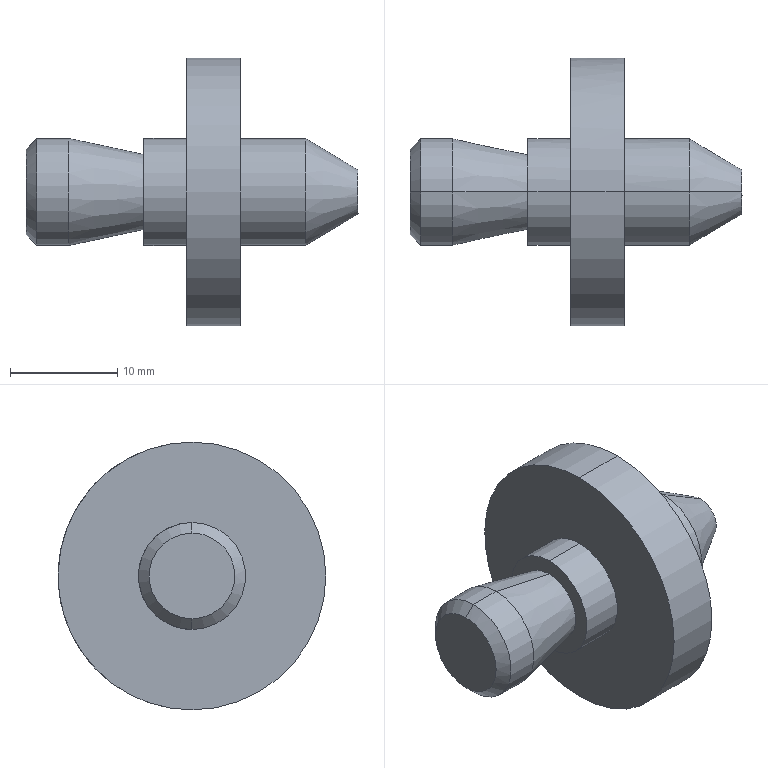Part | STEP file | Positioning_id38_x_t | 1 solid | 19 faces | box 31 x 25 x 25 mm | volume 4152 mm3 | cylinder 8 | cone 6 | plane 5 | commonest cylinder face diameters 10 x6 25 x2
STEP:
#1=CARTESIAN_POINT('',(0.,0.,0.));
#2=DIRECTION('',(0.,0.,1.));
#3=DIRECTION('',(1.,0.,0.));
#4=AXIS2_PLACEMENT_3D('',#1,#2,#3);
#5=CARTESIAN_POINT('',(-829.886,0.00006182,198.532));
#6=VERTEX_POINT('',#5);
#7=CARTESIAN_POINT('',(-824.999,0.00006182,195.6));
#8=VERTEX_POINT('',#7);
#9=CARTESIAN_POINT('',(-824.999,0.00006182,195.6));
#10=DIRECTION('',(0.8575,0.,-0.5145));
#11=VECTOR('',#10,1.);
#12=LINE('',#9,#11);
#13=CARTESIAN_POINT('',(-832.028,0.00006182,193.532));
#14=DIRECTION('',(-1.,0.,0.));
#15=DIRECTION('',(0.,0.,1.));
#16=AXIS2_PLACEMENT_3D('',#13,#14,#15);
#17=CONICAL_SURFACE('',#16,6.285,0.5404);
#18=CARTESIAN_POINT('',(0.,-7.029));
#19=DIRECTION('',(0.,-1.));
#20=VECTOR('',#19,1.);
#21=LINE('',#18,#20);
#22=(GEOMETRIC_REPRESENTATION_CONTEXT(2)PARAMETRIC_REPRESENTATION_CONTEXT()REPRESENTATION_CONTEXT('',''));
#23=DEFINITIONAL_REPRESENTATION('',(#21),#22);
#24=PCURVE('',#17,#23);
#25=CARTESIAN_POINT('',(-832.028,0.00006182,193.532));
#26=DIRECTION('',(-1.,0.,0.));
#27=DIRECTION('',(0.,0.,1.));
#28=AXIS2_PLACEMENT_3D('',#25,#26,#27);
#29=CONICAL_SURFACE('',#28,6.285,0.5404);
#30=CARTESIAN_POINT('',(6.283,-7.029));
#31=DIRECTION('',(0.,-1.));
#32=VECTOR('',#31,1.);
#33=LINE('',#30,#32);
#34=(GEOMETRIC_REPRESENTATION_CONTEXT(2)PARAMETRIC_REPRESENTATION_CONTEXT()REPRESENTATION_CONTEXT('',''));
#35=DEFINITIONAL_REPRESENTATION('',(#33),#34);
#36=PCURVE('',#29,#35);
#37=SURFACE_CURVE('',#12,(#24,#36),.PCURVE_S1.);
#38=EDGE_CURVE('',#6,#8,#37,.T.);
#39=ORIENTED_EDGE('',*,*,#38,.T.);
#40=CARTESIAN_POINT('',(-824.999,0.00006182,191.464));
#41=VERTEX_POINT('',#40);
#42=CARTESIAN_POINT('',(-824.999,0.00006182,193.532));
#43=DIRECTION('',(1.,0.,0.));
#44=DIRECTION('',(0.,0.,1.));
#45=AXIS2_PLACEMENT_3D('',#42,#43,#44);
#46=CIRCLE('',#45,2.068);
#47=CARTESIAN_POINT('',(6.283,-7.029));
#48=DIRECTION('',(-1.,0.));
#49=VECTOR('',#48,1.);
#50=LINE('',#47,#49);
#51=(GEOMETRIC_REPRESENTATION_CONTEXT(2)PARAMETRIC_REPRESENTATION_CONTEXT()REPRESENTATION_CONTEXT('',''));
#52=DEFINITIONAL_REPRESENTATION('',(#50),#51);
#53=PCURVE('',#17,#52);
#54=CARTESIAN_POINT('',(-824.999,0.00006182,193.532));
#55=DIRECTION('',(1.,0.,0.));
#56=DIRECTION('',(0.,0.,1.));
#57=AXIS2_PLACEMENT_3D('',#54,#55,#56);
#58=PLANE('',#57);
#59=CARTESIAN_POINT('',(0.,0.));
#60=DIRECTION('',(1.,0.));
#61=AXIS2_PLACEMENT_2D('',#59,#60);
#62=CIRCLE('',#61,2.068);
#63=(GEOMETRIC_REPRESENTATION_CONTEXT(2)PARAMETRIC_REPRESENTATION_CONTEXT()REPRESENTATION_CONTEXT('',''));
#64=DEFINITIONAL_REPRESENTATION('',(#62),#63);
#65=PCURVE('',#58,#64);
#66=SURFACE_CURVE('',#46,(#53,#65),.PCURVE_S1.);
#67=EDGE_CURVE('',#41,#8,#66,.T.);
#68=ORIENTED_EDGE('',*,*,#67,.F.);
#69=CARTESIAN_POINT('',(-829.886,0.00006182,188.532));
#70=VERTEX_POINT('',#69);
#71=CARTESIAN_POINT('',(-824.999,0.00006182,191.464));
#72=DIRECTION('',(-0.8575,0.,-0.5145));
#73=VECTOR('',#72,1.);
#74=LINE('',#71,#73);
#75=CARTESIAN_POINT('',(3.142,-7.029));
#76=DIRECTION('',(0.,1.));
#77=VECTOR('',#76,1.);
#78=LINE('',#75,#77);
#79=(GEOMETRIC_REPRESENTATION_CONTEXT(2)PARAMETRIC_REPRESENTATION_CONTEXT()REPRESENTATION_CONTEXT('',''));
#80=DEFINITIONAL_REPRESENTATION('',(#78),#79);
#81=PCURVE('',#17,#80);
#82=CARTESIAN_POINT('',(3.142,-7.029));
#83=DIRECTION('',(0.,1.));
#84=VECTOR('',#83,1.);
#85=LINE('',#82,#84);
#86=(GEOMETRIC_REPRESENTATION_CONTEXT(2)PARAMETRIC_REPRESENTATION_CONTEXT()REPRESENTATION_CONTEXT('',''));
#87=DEFINITIONAL_REPRESENTATION('',(#85),#86);
#88=PCURVE('',#29,#87);
#89=SURFACE_CURVE('',#74,(#81,#88),.PCURVE_S1.);
#90=EDGE_CURVE('',#41,#70,#89,.T.);
#91=ORIENTED_EDGE('',*,*,#90,.T.);
#92=CARTESIAN_POINT('',(-829.886,0.00006182,193.532));
#93=DIRECTION('',(-1.,0.,0.));
#94=DIRECTION('',(0.,0.,1.));
#95=AXIS2_PLACEMENT_3D('',#92,#93,#94);
#96=CIRCLE('',#95,5.);
#97=CARTESIAN_POINT('',(0.,-2.142));
#98=DIRECTION('',(1.,0.));
#99=VECTOR('',#98,1.);
#100=LINE('',#97,#99);
#101=(GEOMETRIC_REPRESENTATION_CONTEXT(2)PARAMETRIC_REPRESENTATION_CONTEXT()REPRESENTATION_CONTEXT('',''));
#102=DEFINITIONAL_REPRESENTATION('',(#100),#101);
#103=PCURVE('',#17,#102);
#104=CARTESIAN_POINT('',(-835.999,0.00006182,193.532));
#105=DIRECTION('',(-1.,0.,0.));
#106=DIRECTION('',(0.,0.,1.));
#107=AXIS2_PLACEMENT_3D('',#104,#105,#106);
#108=CYLINDRICAL_SURFACE('',#107,5.);
#109=CARTESIAN_POINT('',(0.,-6.113));
#110=DIRECTION('',(1.,0.));
#111=VECTOR('',#110,1.);
#112=LINE('',#109,#111);
#113=(GEOMETRIC_REPRESENTATION_CONTEXT(2)PARAMETRIC_REPRESENTATION_CONTEXT()REPRESENTATION_CONTEXT('',''));
#114=DEFINITIONAL_REPRESENTATION('',(#112),#113);
#115=PCURVE('',#108,#114);
#116=SURFACE_CURVE('',#96,(#103,#115),.PCURVE_S1.);
#117=EDGE_CURVE('',#6,#70,#116,.T.);
#118=ORIENTED_EDGE('',*,*,#117,.F.);
#119=EDGE_LOOP('',(#39,#68,#91,#118));
#120=FACE_BOUND('',#119,.T.);
#121=ADVANCED_FACE('',(#120),#17,.T.);
#122=CARTESIAN_POINT('',(-835.999,0.00006182,198.532));
#123=VERTEX_POINT('',#122);
#124=CARTESIAN_POINT('',(-835.999,0.00006182,198.532));
#125=DIRECTION('',(1.,0.,0.));
#126=VECTOR('',#125,1.);
#127=LINE('',#124,#126);
#128=CARTESIAN_POINT('',(-835.999,0.00006182,193.532));
#129=DIRECTION('',(-1.,0.,0.));
#130=DIRECTION('',(0.,0.,1.));
#131=AXIS2_PLACEMENT_3D('',#128,#129,#130);
#132=CYLINDRICAL_SURFACE('',#131,5.);
#133=CARTESIAN_POINT('',(6.283,0.));
#134=DIRECTION('',(0.,-1.));
#135=VECTOR('',#134,1.);
#136=LINE('',#133,#135);
#137=(GEOMETRIC_REPRESENTATION_CONTEXT(2)PARAMETRIC_REPRESENTATION_CONTEXT()REPRESENTATION_CONTEXT('',''));
#138=DEFINITIONAL_REPRESENTATION('',(#136),#137);
#139=PCURVE('',#132,#138);
#140=CARTESIAN_POINT('',(0.,0.));
#141=DIRECTION('',(0.,-1.));
#142=VECTOR('',#141,1.);
#143=LINE('',#140,#142);
#144=(GEOMETRIC_REPRESENTATION_CONTEXT(2)PARAMETRIC_REPRESENTATION_CONTEXT()REPRESENTATION_CONTEXT('',''));
#145=DEFINITIONAL_REPRESENTATION('',(#143),#144);
#146=PCURVE('',#108,#145);
#147=SURFACE_CURVE('',#127,(#139,#146),.PCURVE_S1.);
#148=EDGE_CURVE('',#123,#6,#147,.T.);
#149=ORIENTED_EDGE('',*,*,#148,.F.);
#150=CARTESIAN_POINT('',(-835.999,0.00006182,188.532));
#151=VERTEX_POINT('',#150);
#152=CARTESIAN_POINT('',(-835.999,0.00006182,193.532));
#153=DIRECTION('',(1.,0.,0.));
#154=DIRECTION('',(0.,0.,1.));
#155=AXIS2_PLACEMENT_3D('',#152,#153,#154);
#156=CIRCLE('',#155,5.);
#157=CARTESIAN_POINT('',(6.283,0.));
#158=DIRECTION('',(-1.,0.));
#159=VECTOR('',#158,1.);
#160=LINE('',#157,#159);
#161=(GEOMETRIC_REPRESENTATION_CONTEXT(2)PARAMETRIC_REPRESENTATION_CONTEXT()REPRESENTATION_CONTEXT('',''));
#162=DEFINITIONAL_REPRESENTATION('',(#160),#161);
#163=PCURVE('',#132,#162);
#164=CARTESIAN_POINT('',(-835.999,0.00006182,193.532));
#165=DIRECTION('',(1.,0.,0.));
#166=DIRECTION('',(0.,0.,1.));
#167=AXIS2_PLACEMENT_3D('',#164,#165,#166);
#168=PLANE('',#167);
#169=CARTESIAN_POINT('',(0.,0.));
#170=DIRECTION('',(1.,0.));
#171=AXIS2_PLACEMENT_2D('',#169,#170);
#172=CIRCLE('',#171,5.);
#173=(GEOMETRIC_REPRESENTATION_CONTEXT(2)PARAMETRIC_REPRESENTATION_CONTEXT()REPRESENTATION_CONTEXT('',''));
#174=DEFINITIONAL_REPRESENTATION('',(#172),#173);
#175=PCURVE('',#168,#174);
#176=SURFACE_CURVE('',#156,(#163,#175),.PCURVE_S1.);
#177=EDGE_CURVE('',#123,#151,#176,.T.);
#178=ORIENTED_EDGE('',*,*,#177,.T.);
#179=CARTESIAN_POINT('',(-835.999,0.00006182,188.532));
#180=DIRECTION('',(-1.,0.,0.));
#181=VECTOR('',#180,1.);
#182=LINE('',#179,#181);
#183=CARTESIAN_POINT('',(3.142,0.));
#184=DIRECTION('',(0.,1.));
#185=VECTOR('',#184,1.);
#186=LINE('',#183,#185);
#187=(GEOMETRIC_REPRESENTATION_CONTEXT(2)PARAMETRIC_REPRESENTATION_CONTEXT()REPRESENTATION_CONTEXT('',''));
#188=DEFINITIONAL_REPRESENTATION('',(#186),#187);
#189=PCURVE('',#132,#188);
#190=CARTESIAN_POINT('',(3.142,0.));
#191=DIRECTION('',(0.,1.));
#192=VECTOR('',#191,1.);
#193=LINE('',#190,#192);
#194=(GEOMETRIC_REPRESENTATION_CONTEXT(2)PARAMETRIC_REPRESENTATION_CONTEXT()REPRESENTATION_CONTEXT('',''));
#195=DEFINITIONAL_REPRESENTATION('',(#193),#194);
#196=PCURVE('',#108,#195);
#197=SURFACE_CURVE('',#182,(#189,#196),.PCURVE_S1.);
#198=EDGE_CURVE('',#70,#151,#197,.T.);
#199=ORIENTED_EDGE('',*,*,#198,.F.);
#200=CARTESIAN_POINT('',(-829.886,0.00006182,193.532));
#201=DIRECTION('',(-1.,0.,0.));
#202=DIRECTION('',(0.,0.,-1.));
#203=AXIS2_PLACEMENT_3D('',#200,#201,#202);
#204=CIRCLE('',#203,5.);
#205=CARTESIAN_POINT('',(3.142,-6.113));
#206=DIRECTION('',(1.,0.));
#207=VECTOR('',#206,1.);
#208=LINE('',#205,#207);
#209=(GEOMETRIC_REPRESENTATION_CONTEXT(2)PARAMETRIC_REPRESENTATION_CONTEXT()REPRESENTATION_CONTEXT('',''));
#210=DEFINITIONAL_REPRESENTATION('',(#208),#209);
#211=PCURVE('',#132,#210);
#212=CARTESIAN_POINT('',(3.142,-2.142));
#213=DIRECTION('',(1.,0.));
#214=VECTOR('',#213,1.);
#215=LINE('',#212,#214);
#216=(GEOMETRIC_REPRESENTATION_CONTEXT(2)PARAMETRIC_REPRESENTATION_CONTEXT()REPRESENTATION_CONTEXT('',''));
#217=DEFINITIONAL_REPRESENTATION('',(#215),#216);
#218=PCURVE('',#29,#217);
#219=SURFACE_CURVE('',#204,(#211,#218),.PCURVE_S1.);
#220=EDGE_CURVE('',#70,#6,#219,.T.);
#221=ORIENTED_EDGE('',*,*,#220,.T.);
#222=EDGE_LOOP('',(#149,#178,#199,#221));
#223=FACE_BOUND('',#222,.T.);
#224=ADVANCED_FACE('',(#223),#132,.T.);
#225=ORIENTED_EDGE('',*,*,#67,.T.);
#226=CARTESIAN_POINT('',(-824.999,0.00006182,195.6));
#227=CARTESIAN_POINT('',(-824.999,-2.068,195.6));
#228=CARTESIAN_POINT('',(-824.999,-3.101,193.532));
#229=CARTESIAN_POINT('',(-824.999,-2.068,191.464));
#230=CARTESIAN_POINT('',(-824.999,0.00006182,191.464));
#231=(BOUNDED_CURVE()B_SPLINE_CURVE(4,(#226,#227,#228,#229,#230),.UNSPECIFIED.,.F.,.F.)B_SPLINE_CURVE_WITH_KNOTS((5,5),(0.,1.),.PIECEWISE_BEZIER_KNOTS.)CURVE()GEOMETRIC_REPRESENTATION_ITEM()RATIONAL_B_SPLINE_CURVE((1.,0.7071,0.6667,0.7071,1.))REPRESENTATION_ITEM(''));
#232=CARTESIAN_POINT('',(2.068,0.));
#233=CARTESIAN_POINT('',(2.068,2.068));
#234=CARTESIAN_POINT('',(0.,3.101));
#235=CARTESIAN_POINT('',(-2.068,2.068));
#236=CARTESIAN_POINT('',(-2.068,0.));
#237=(BOUNDED_CURVE()B_SPLINE_CURVE(4,(#232,#233,#234,#235,#236),.UNSPECIFIED.,.F.,.F.)B_SPLINE_CURVE_WITH_KNOTS((5,5),(0.,1.),.PIECEWISE_BEZIER_KNOTS.)CURVE()GEOMETRIC_REPRESENTATION_ITEM()RATIONAL_B_SPLINE_CURVE((1.,0.7071,0.6667,0.7071,1.))REPRESENTATION_ITEM(''));
#238=(GEOMETRIC_REPRESENTATION_CONTEXT(2)PARAMETRIC_REPRESENTATION_CONTEXT()REPRESENTATION_CONTEXT('',''));
#239=DEFINITIONAL_REPRESENTATION('',(#237),#238);
#240=PCURVE('',#58,#239);
#241=CARTESIAN_POINT('',(6.283,-7.029));
#242=CARTESIAN_POINT('',(6.24,-7.029));
#243=CARTESIAN_POINT('',(6.153,-7.029));
#244=CARTESIAN_POINT('',(6.02,-7.029));
#245=CARTESIAN_POINT('',(5.883,-7.029));
#246=CARTESIAN_POINT('',(5.744,-7.029));
#247=CARTESIAN_POINT('',(5.602,-7.029));
#248=CARTESIAN_POINT('',(5.457,-7.029));
#249=CARTESIAN_POINT('',(5.311,-7.029));
#250=CARTESIAN_POINT('',(5.163,-7.029));
#251=CARTESIAN_POINT('',(5.013,-7.029));
#252=CARTESIAN_POINT('',(4.863,-7.029));
#253=CARTESIAN_POINT('',(4.712,-7.029));
#254=CARTESIAN_POINT('',(4.562,-7.029));
#255=CARTESIAN_POINT('',(4.412,-7.029));
#256=CARTESIAN_POINT('',(4.262,-7.029));
#257=CARTESIAN_POINT('',(4.114,-7.029));
#258=CARTESIAN_POINT('',(3.968,-7.029));
#259=CARTESIAN_POINT('',(3.823,-7.029));
#260=CARTESIAN_POINT('',(3.681,-7.029));
#261=CARTESIAN_POINT('',(3.542,-7.029));
#262=CARTESIAN_POINT('',(3.405,-7.029));
#263=CARTESIAN_POINT('',(3.271,-7.029));
#264=CARTESIAN_POINT('',(3.184,-7.029));
#265=CARTESIAN_POINT('',(3.142,-7.029));
#266=B_SPLINE_CURVE_WITH_KNOTS('',3,(#241,#242,#243,#244,#245,#246,#247,#248,#249,#250,#251,#252,#253,#254,#255,#256,#257,#258,#259,#260,#261,#262,#263,#264,#265),.UNSPECIFIED.,.F.,.F.,(4,1,1,1,1,1,1,1,1,1,1,1,1,1,1,1,1,1,1,1,1,1,4),(0.,0.04545,0.09091,0.1364,0.1818,0.2273,0.2727,0.3182,0.3636,0.4091,0.4545,0.5,0.5455,0.5909,0.6364,0.6818,0.7273,0.7727,0.8182,0.8636,0.9091,0.9545,1.),.QUASI_UNIFORM_KNOTS.);
#267=(GEOMETRIC_REPRESENTATION_CONTEXT(2)PARAMETRIC_REPRESENTATION_CONTEXT()REPRESENTATION_CONTEXT('',''));
#268=DEFINITIONAL_REPRESENTATION('',(#266),#267);
#269=PCURVE('',#29,#268);
#270=SURFACE_CURVE('',#231,(#240,#269),.PCURVE_S1.);
#271=EDGE_CURVE('',#8,#41,#270,.T.);
#272=ORIENTED_EDGE('',*,*,#271,.T.);
#273=EDGE_LOOP('',(#225,#272));
#274=FACE_BOUND('',#273,.T.);
#275=ADVANCED_FACE('',(#274),#58,.T.);
#276=CARTESIAN_POINT('',(-844.999,0.00006182,190.032));
#277=VERTEX_POINT('',#276);
#278=CARTESIAN_POINT('',(-844.999,0.00006182,197.032));
#279=VERTEX_POINT('',#278);
#280=CARTESIAN_POINT('',(-844.999,0.00006182,193.532));
#281=DIRECTION('',(1.,0.,0.));
#282=DIRECTION('',(0.,0.,-1.));
#283=AXIS2_PLACEMENT_3D('',#280,#281,#282);
#284=CIRCLE('',#283,3.5);
#285=CARTESIAN_POINT('',(-844.999,0.00006182,193.532));
#286=DIRECTION('',(1.,0.,0.));
#287=DIRECTION('',(0.,0.,1.));
#288=AXIS2_PLACEMENT_3D('',#285,#286,#287);
#289=PLANE('',#288);
#290=CARTESIAN_POINT('',(0.,0.));
#291=DIRECTION('',(-1.,0.));
#292=AXIS2_PLACEMENT_2D('',#290,#291);
#293=CIRCLE('',#292,3.5);
#294=(GEOMETRIC_REPRESENTATION_CONTEXT(2)PARAMETRIC_REPRESENTATION_CONTEXT()REPRESENTATION_CONTEXT('',''));
#295=DEFINITIONAL_REPRESENTATION('',(#293),#294);
#296=PCURVE('',#289,#295);
#297=CARTESIAN_POINT('',(-851.999,0.00006182,193.532));
#298=DIRECTION('',(-1.,0.,0.));
#299=DIRECTION('',(0.,0.,1.));
#300=AXIS2_PLACEMENT_3D('',#297,#298,#299);
#301=CONICAL_SURFACE('',#300,5.,0.2111);
#302=CARTESIAN_POINT('',(3.142,-7.));
#303=DIRECTION('',(-1.,0.));
#304=VECTOR('',#303,1.);
#305=LINE('',#302,#304);
#306=(GEOMETRIC_REPRESENTATION_CONTEXT(2)PARAMETRIC_REPRESENTATION_CONTEXT()REPRESENTATION_CONTEXT('',''));
#307=DEFINITIONAL_REPRESENTATION('',(#305),#306);
#308=PCURVE('',#301,#307);
#309=SURFACE_CURVE('',#284,(#296,#308),.PCURVE_S1.);
#310=EDGE_CURVE('',#277,#279,#309,.T.);
#311=ORIENTED_EDGE('',*,*,#310,.T.);
#312=CARTESIAN_POINT('',(-844.999,0.00006182,193.532));
#313=DIRECTION('',(1.,0.,0.));
#314=DIRECTION('',(0.,0.,1.));
#315=AXIS2_PLACEMENT_3D('',#312,#313,#314);
#316=CIRCLE('',#315,3.5);
#317=CARTESIAN_POINT('',(0.,0.));
#318=DIRECTION('',(1.,0.));
#319=AXIS2_PLACEMENT_2D('',#317,#318);
#320=CIRCLE('',#319,3.5);
#321=(GEOMETRIC_REPRESENTATION_CONTEXT(2)PARAMETRIC_REPRESENTATION_CONTEXT()REPRESENTATION_CONTEXT('',''));
#322=DEFINITIONAL_REPRESENTATION('',(#320),#321);
#323=PCURVE('',#289,#322);
#324=CARTESIAN_POINT('',(-851.999,0.00006182,193.532));
#325=DIRECTION('',(-1.,0.,0.));
#326=DIRECTION('',(0.,0.,1.));
#327=AXIS2_PLACEMENT_3D('',#324,#325,#326);
#328=CONICAL_SURFACE('',#327,5.,0.2111);
#329=CARTESIAN_POINT('',(6.283,-7.));
#330=DIRECTION('',(-1.,0.));
#331=VECTOR('',#330,1.);
#332=LINE('',#329,#331);
#333=(GEOMETRIC_REPRESENTATION_CONTEXT(2)PARAMETRIC_REPRESENTATION_CONTEXT()REPRESENTATION_CONTEXT('',''));
#334=DEFINITIONAL_REPRESENTATION('',(#332),#333);
#335=PCURVE('',#328,#334);
#336=SURFACE_CURVE('',#316,(#323,#335),.PCURVE_S1.);
#337=EDGE_CURVE('',#279,#277,#336,.T.);
#338=ORIENTED_EDGE('',*,*,#337,.T.);
#339=EDGE_LOOP('',(#311,#338));
#340=FACE_BOUND('',#339,.T.);
#341=CARTESIAN_POINT('',(-844.999,0.00006182,188.532));
#342=VERTEX_POINT('',#341);
#343=CARTESIAN_POINT('',(-844.999,0.00006182,198.532));
#344=VERTEX_POINT('',#343);
#345=CARTESIAN_POINT('',(-844.999,0.00006182,193.532));
#346=DIRECTION('',(-1.,0.,0.));
#347=DIRECTION('',(0.,0.,-1.));
#348=AXIS2_PLACEMENT_3D('',#345,#346,#347);
#349=CIRCLE('',#348,5.);
#350=CARTESIAN_POINT('',(-5.,0.));
#351=CARTESIAN_POINT('',(-5.,8.66));
#352=CARTESIAN_POINT('',(2.5,4.33));
#353=CARTESIAN_POINT('',(10.,0.));
#354=CARTESIAN_POINT('',(2.5,-4.33));
#355=CARTESIAN_POINT('',(-5.,-8.66));
#356=CARTESIAN_POINT('',(-5.,0.));
#357=(BOUNDED_CURVE()B_SPLINE_CURVE(2,(#350,#351,#352,#353,#354,#355,#356),.UNSPECIFIED.,.T.,.F.)B_SPLINE_CURVE_WITH_KNOTS((1,2,2,2,2,1),(-2.094,0.,2.094,4.189,6.283,8.378),.UNSPECIFIED.)CURVE()GEOMETRIC_REPRESENTATION_ITEM()RATIONAL_B_SPLINE_CURVE((1.,0.5,1.,0.5,1.,0.5,1.))REPRESENTATION_ITEM(''));
#358=(GEOMETRIC_REPRESENTATION_CONTEXT(2)PARAMETRIC_REPRESENTATION_CONTEXT()REPRESENTATION_CONTEXT('',''));
#359=DEFINITIONAL_REPRESENTATION('',(#357),#358);
#360=PCURVE('',#289,#359);
#361=CARTESIAN_POINT('',(-845.999,0.00006182,193.532));
#362=DIRECTION('',(-1.,0.,0.));
#363=DIRECTION('',(0.,0.,1.));
#364=AXIS2_PLACEMENT_3D('',#361,#362,#363);
#365=CYLINDRICAL_SURFACE('',#364,5.);
#366=CARTESIAN_POINT('',(3.142,-1.));
#367=DIRECTION('',(1.,0.));
#368=VECTOR('',#367,1.);
#369=LINE('',#366,#368);
#370=(GEOMETRIC_REPRESENTATION_CONTEXT(2)PARAMETRIC_REPRESENTATION_CONTEXT()REPRESENTATION_CONTEXT('',''));
#371=DEFINITIONAL_REPRESENTATION('',(#369),#370);
#372=PCURVE('',#365,#371);
#373=SURFACE_CURVE('',#349,(#360,#372),.PCURVE_S1.);
#374=EDGE_CURVE('',#342,#344,#373,.T.);
#375=ORIENTED_EDGE('',*,*,#374,.T.);
#376=CARTESIAN_POINT('',(-844.999,0.00006182,193.532));
#377=DIRECTION('',(-1.,0.,0.));
#378=DIRECTION('',(0.,0.,1.));
#379=AXIS2_PLACEMENT_3D('',#376,#377,#378);
#380=CIRCLE('',#379,5.);
#381=CARTESIAN_POINT('',(5.,0.));
#382=CARTESIAN_POINT('',(5.,-8.66));
#383=CARTESIAN_POINT('',(-2.5,-4.33));
#384=CARTESIAN_POINT('',(-10.,0.));
#385=CARTESIAN_POINT('',(-2.5,4.33));
#386=CARTESIAN_POINT('',(5.,8.66));
#387=CARTESIAN_POINT('',(5.,0.));
#388=(BOUNDED_CURVE()B_SPLINE_CURVE(2,(#381,#382,#383,#384,#385,#386,#387),.UNSPECIFIED.,.T.,.F.)B_SPLINE_CURVE_WITH_KNOTS((1,2,2,2,2,1),(-2.094,0.,2.094,4.189,6.283,8.378),.UNSPECIFIED.)CURVE()GEOMETRIC_REPRESENTATION_ITEM()RATIONAL_B_SPLINE_CURVE((1.,0.5,1.,0.5,1.,0.5,1.))REPRESENTATION_ITEM(''));
#389=(GEOMETRIC_REPRESENTATION_CONTEXT(2)PARAMETRIC_REPRESENTATION_CONTEXT()REPRESENTATION_CONTEXT('',''));
#390=DEFINITIONAL_REPRESENTATION('',(#388),#389);
#391=PCURVE('',#289,#390);
#392=CARTESIAN_POINT('',(-845.999,0.00006182,193.532));
#393=DIRECTION('',(-1.,0.,0.));
#394=DIRECTION('',(0.,0.,1.));
#395=AXIS2_PLACEMENT_3D('',#392,#393,#394);
#396=CYLINDRICAL_SURFACE('',#395,5.);
#397=CARTESIAN_POINT('',(0.,-1.));
#398=DIRECTION('',(1.,0.));
#399=VECTOR('',#398,1.);
#400=LINE('',#397,#399);
#401=(GEOMETRIC_REPRESENTATION_CONTEXT(2)PARAMETRIC_REPRESENTATION_CONTEXT()REPRESENTATION_CONTEXT('',''));
#402=DEFINITIONAL_REPRESENTATION('',(#400),#401);
#403=PCURVE('',#396,#402);
#404=SURFACE_CURVE('',#380,(#391,#403),.PCURVE_S1.);
#405=EDGE_CURVE('',#344,#342,#404,.T.);
#406=ORIENTED_EDGE('',*,*,#405,.T.);
#407=EDGE_LOOP('',(#375,#406));
#408=FACE_BOUND('',#407,.T.);
#409=ADVANCED_FACE('',(#340,#408),#289,.F.);
#410=CARTESIAN_POINT('',(-840.999,0.00006182,198.532));
#411=VERTEX_POINT('',#410);
#412=CARTESIAN_POINT('',(-844.999,0.00006182,198.532));
#413=DIRECTION('',(-1.,0.,0.));
#414=VECTOR('',#413,1.);
#415=LINE('',#412,#414);
#416=CARTESIAN_POINT('',(6.283,-1.));
#417=DIRECTION('',(0.,1.));
#418=VECTOR('',#417,1.);
#419=LINE('',#416,#418);
#420=(GEOMETRIC_REPRESENTATION_CONTEXT(2)PARAMETRIC_REPRESENTATION_CONTEXT()REPRESENTATION_CONTEXT('',''));
#421=DEFINITIONAL_REPRESENTATION('',(#419),#420);
#422=PCURVE('',#365,#421);
#423=CARTESIAN_POINT('',(0.,-1.));
#424=DIRECTION('',(0.,1.));
#425=VECTOR('',#424,1.);
#426=LINE('',#423,#425);
#427=(GEOMETRIC_REPRESENTATION_CONTEXT(2)PARAMETRIC_REPRESENTATION_CONTEXT()REPRESENTATION_CONTEXT('',''));
#428=DEFINITIONAL_REPRESENTATION('',(#426),#427);
#429=PCURVE('',#396,#428);
#430=SURFACE_CURVE('',#415,(#422,#429),.PCURVE_S1.);
#431=EDGE_CURVE('',#411,#344,#430,.T.);
#432=ORIENTED_EDGE('',*,*,#431,.T.);
#433=ORIENTED_EDGE('',*,*,#374,.F.);
#434=CARTESIAN_POINT('',(-840.999,0.00006182,188.532));
#435=VERTEX_POINT('',#434);
#436=CARTESIAN_POINT('',(-844.999,0.00006182,188.532));
#437=DIRECTION('',(1.,0.,0.));
#438=VECTOR('',#437,1.);
#439=LINE('',#436,#438);
#440=CARTESIAN_POINT('',(3.142,-1.));
#441=DIRECTION('',(0.,-1.));
#442=VECTOR('',#441,1.);
#443=LINE('',#440,#442);
#444=(GEOMETRIC_REPRESENTATION_CONTEXT(2)PARAMETRIC_REPRESENTATION_CONTEXT()REPRESENTATION_CONTEXT('',''));
#445=DEFINITIONAL_REPRESENTATION('',(#443),#444);
#446=PCURVE('',#365,#445);
#447=CARTESIAN_POINT('',(3.142,-1.));
#448=DIRECTION('',(0.,-1.));
#449=VECTOR('',#448,1.);
#450=LINE('',#447,#449);
#451=(GEOMETRIC_REPRESENTATION_CONTEXT(2)PARAMETRIC_REPRESENTATION_CONTEXT()REPRESENTATION_CONTEXT('',''));
#452=DEFINITIONAL_REPRESENTATION('',(#450),#451);
#453=PCURVE('',#396,#452);
#454=SURFACE_CURVE('',#439,(#446,#453),.PCURVE_S1.);
#455=EDGE_CURVE('',#342,#435,#454,.T.);
#456=ORIENTED_EDGE('',*,*,#455,.T.);
#457=CARTESIAN_POINT('',(-840.999,0.00006182,193.532));
#458=DIRECTION('',(-1.,0.,0.));
#459=DIRECTION('',(0.,0.,1.));
#460=AXIS2_PLACEMENT_3D('',#457,#458,#459);
#461=CIRCLE('',#460,5.);
#462=CARTESIAN_POINT('',(0.,-5.));
#463=DIRECTION('',(1.,0.));
#464=VECTOR('',#463,1.);
#465=LINE('',#462,#464);
#466=(GEOMETRIC_REPRESENTATION_CONTEXT(2)PARAMETRIC_REPRESENTATION_CONTEXT()REPRESENTATION_CONTEXT('',''));
#467=DEFINITIONAL_REPRESENTATION('',(#465),#466);
#468=PCURVE('',#365,#467);
#469=CARTESIAN_POINT('',(-840.999,0.00006182,193.532));
#470=DIRECTION('',(-1.,0.,0.));
#471=DIRECTION('',(0.,0.,-1.));
#472=AXIS2_PLACEMENT_3D('',#469,#470,#471);
#473=PLANE('',#472);
#474=CARTESIAN_POINT('',(0.,0.));
#475=DIRECTION('',(-1.,0.));
#476=AXIS2_PLACEMENT_2D('',#474,#475);
#477=CIRCLE('',#476,5.);
#478=(GEOMETRIC_REPRESENTATION_CONTEXT(2)PARAMETRIC_REPRESENTATION_CONTEXT()REPRESENTATION_CONTEXT('',''));
#479=DEFINITIONAL_REPRESENTATION('',(#477),#478);
#480=PCURVE('',#473,#479);
#481=SURFACE_CURVE('',#461,(#468,#480),.PCURVE_S1.);
#482=EDGE_CURVE('',#435,#411,#481,.T.);
#483=ORIENTED_EDGE('',*,*,#482,.T.);
#484=EDGE_LOOP('',(#432,#433,#456,#483));
#485=FACE_BOUND('',#484,.T.);
#486=ADVANCED_FACE('',(#485),#365,.T.);
#487=CARTESIAN_POINT('',(-851.999,0.00006182,198.532));
#488=VERTEX_POINT('',#487);
#489=CARTESIAN_POINT('',(-844.999,0.00006182,197.032));
#490=DIRECTION('',(0.9778,0.,-0.2095));
#491=VECTOR('',#490,1.);
#492=LINE('',#489,#491);
#493=CARTESIAN_POINT('',(0.,-7.));
#494=DIRECTION('',(0.,-1.));
#495=VECTOR('',#494,1.);
#496=LINE('',#493,#495);
#497=(GEOMETRIC_REPRESENTATION_CONTEXT(2)PARAMETRIC_REPRESENTATION_CONTEXT()REPRESENTATION_CONTEXT('',''));
#498=DEFINITIONAL_REPRESENTATION('',(#496),#497);
#499=PCURVE('',#301,#498);
#500=CARTESIAN_POINT('',(6.283,-7.));
#501=DIRECTION('',(0.,-1.));
#502=VECTOR('',#501,1.);
#503=LINE('',#500,#502);
#504=(GEOMETRIC_REPRESENTATION_CONTEXT(2)PARAMETRIC_REPRESENTATION_CONTEXT()REPRESENTATION_CONTEXT('',''));
#505=DEFINITIONAL_REPRESENTATION('',(#503),#504);
#506=PCURVE('',#328,#505);
#507=SURFACE_CURVE('',#492,(#499,#506),.PCURVE_S1.);
#508=EDGE_CURVE('',#488,#279,#507,.T.);
#509=ORIENTED_EDGE('',*,*,#508,.T.);
#510=ORIENTED_EDGE('',*,*,#310,.F.);
#511=CARTESIAN_POINT('',(-851.999,0.00006182,188.532));
#512=VERTEX_POINT('',#511);
#513=CARTESIAN_POINT('',(-844.999,0.00006182,190.032));
#514=DIRECTION('',(-0.9778,0.,-0.2095));
#515=VECTOR('',#514,1.);
#516=LINE('',#513,#515);
#517=CARTESIAN_POINT('',(3.142,-7.));
#518=DIRECTION('',(0.,1.));
#519=VECTOR('',#518,1.);
#520=LINE('',#517,#519);
#521=(GEOMETRIC_REPRESENTATION_CONTEXT(2)PARAMETRIC_REPRESENTATION_CONTEXT()REPRESENTATION_CONTEXT('',''));
#522=DEFINITIONAL_REPRESENTATION('',(#520),#521);
#523=PCURVE('',#301,#522);
#524=CARTESIAN_POINT('',(3.142,-7.));
#525=DIRECTION('',(0.,1.));
#526=VECTOR('',#525,1.);
#527=LINE('',#524,#526);
#528=(GEOMETRIC_REPRESENTATION_CONTEXT(2)PARAMETRIC_REPRESENTATION_CONTEXT()REPRESENTATION_CONTEXT('',''));
#529=DEFINITIONAL_REPRESENTATION('',(#527),#528);
#530=PCURVE('',#328,#529);
#531=SURFACE_CURVE('',#516,(#523,#530),.PCURVE_S1.);
#532=EDGE_CURVE('',#277,#512,#531,.T.);
#533=ORIENTED_EDGE('',*,*,#532,.T.);
#534=CARTESIAN_POINT('',(-851.999,0.00006182,193.532));
#535=DIRECTION('',(-1.,0.,0.));
#536=DIRECTION('',(0.,0.,1.));
#537=AXIS2_PLACEMENT_3D('',#534,#535,#536);
#538=CIRCLE('',#537,5.);
#539=CARTESIAN_POINT('',(0.,0.));
#540=DIRECTION('',(1.,0.));
#541=VECTOR('',#540,1.);
#542=LINE('',#539,#541);
#543=(GEOMETRIC_REPRESENTATION_CONTEXT(2)PARAMETRIC_REPRESENTATION_CONTEXT()REPRESENTATION_CONTEXT('',''));
#544=DEFINITIONAL_REPRESENTATION('',(#542),#543);
#545=PCURVE('',#301,#544);
#546=CARTESIAN_POINT('',(-845.999,0.00006182,193.532));
#547=DIRECTION('',(-1.,0.,0.));
#548=DIRECTION('',(0.,0.,1.));
#549=AXIS2_PLACEMENT_3D('',#546,#547,#548);
#550=CYLINDRICAL_SURFACE('',#549,5.);
#551=CARTESIAN_POINT('',(0.,6.));
#552=DIRECTION('',(1.,0.));
#553=VECTOR('',#552,1.);
#554=LINE('',#551,#553);
#555=(GEOMETRIC_REPRESENTATION_CONTEXT(2)PARAMETRIC_REPRESENTATION_CONTEXT()REPRESENTATION_CONTEXT('',''));
#556=DEFINITIONAL_REPRESENTATION('',(#554),#555);
#557=PCURVE('',#550,#556);
#558=SURFACE_CURVE('',#538,(#545,#557),.PCURVE_S1.);
#559=EDGE_CURVE('',#488,#512,#558,.T.);
#560=ORIENTED_EDGE('',*,*,#559,.F.);
#561=EDGE_LOOP('',(#509,#510,#533,#560));
#562=FACE_BOUND('',#561,.T.);
#563=ADVANCED_FACE('',(#562),#301,.T.);
#564=CARTESIAN_POINT('',(-854.999,0.00006182,188.532));
#565=VERTEX_POINT('',#564);
#566=CARTESIAN_POINT('',(-855.999,0.00006182,189.532));
#567=VERTEX_POINT('',#566);
#568=CARTESIAN_POINT('',(-855.999,0.00006182,189.532));
#569=DIRECTION('',(-0.7071,0.,0.7071));
#570=VECTOR('',#569,1.);
#571=LINE('',#568,#570);
#572=CARTESIAN_POINT('',(-854.999,0.00006182,193.532));
#573=DIRECTION('',(1.,0.,0.));
#574=DIRECTION('',(0.,0.,-1.));
#575=AXIS2_PLACEMENT_3D('',#572,#573,#574);
#576=CONICAL_SURFACE('',#575,5.,0.7854);
#577=CARTESIAN_POINT('',(0.,-1.));
#578=DIRECTION('',(0.,-1.));
#579=VECTOR('',#578,1.);
#580=LINE('',#577,#579);
#581=(GEOMETRIC_REPRESENTATION_CONTEXT(2)PARAMETRIC_REPRESENTATION_CONTEXT()REPRESENTATION_CONTEXT('',''));
#582=DEFINITIONAL_REPRESENTATION('',(#580),#581);
#583=PCURVE('',#576,#582);
#584=CARTESIAN_POINT('',(-854.999,0.00006182,193.532));
#585=DIRECTION('',(1.,0.,0.));
#586=DIRECTION('',(0.,0.,-1.));
#587=AXIS2_PLACEMENT_3D('',#584,#585,#586);
#588=CONICAL_SURFACE('',#587,5.,0.7854);
#589=CARTESIAN_POINT('',(6.283,-1.));
#590=DIRECTION('',(0.,-1.));
#591=VECTOR('',#590,1.);
#592=LINE('',#589,#591);
#593=(GEOMETRIC_REPRESENTATION_CONTEXT(2)PARAMETRIC_REPRESENTATION_CONTEXT()REPRESENTATION_CONTEXT('',''));
#594=DEFINITIONAL_REPRESENTATION('',(#592),#593);
#595=PCURVE('',#588,#594);
#596=SURFACE_CURVE('',#571,(#583,#595),.PCURVE_S1.);
#597=EDGE_CURVE('',#565,#567,#596,.T.);
#598=ORIENTED_EDGE('',*,*,#597,.T.);
#599=CARTESIAN_POINT('',(-855.999,0.00006182,197.532));
#600=VERTEX_POINT('',#599);
#601=CARTESIAN_POINT('',(-855.999,0.00006182,193.532));
#602=DIRECTION('',(-1.,0.,0.));
#603=DIRECTION('',(0.,0.,-1.));
#604=AXIS2_PLACEMENT_3D('',#601,#602,#603);
#605=CIRCLE('',#604,4.);
#606=CARTESIAN_POINT('',(6.283,-1.));
#607=DIRECTION('',(-1.,0.));
#608=VECTOR('',#607,1.);
#609=LINE('',#606,#608);
#610=(GEOMETRIC_REPRESENTATION_CONTEXT(2)PARAMETRIC_REPRESENTATION_CONTEXT()REPRESENTATION_CONTEXT('',''));
#611=DEFINITIONAL_REPRESENTATION('',(#609),#610);
#612=PCURVE('',#576,#611);
#613=CARTESIAN_POINT('',(-855.999,0.00006182,193.532));
#614=DIRECTION('',(-1.,0.,0.));
#615=DIRECTION('',(0.,0.,-1.));
#616=AXIS2_PLACEMENT_3D('',#613,#614,#615);
#617=PLANE('',#616);
#618=CARTESIAN_POINT('',(0.,0.));
#619=DIRECTION('',(1.,0.));
#620=AXIS2_PLACEMENT_2D('',#618,#619);
#621=CIRCLE('',#620,4.);
#622=(GEOMETRIC_REPRESENTATION_CONTEXT(2)PARAMETRIC_REPRESENTATION_CONTEXT()REPRESENTATION_CONTEXT('',''));
#623=DEFINITIONAL_REPRESENTATION('',(#621),#622);
#624=PCURVE('',#617,#623);
#625=SURFACE_CURVE('',#605,(#612,#624),.PCURVE_S1.);
#626=EDGE_CURVE('',#600,#567,#625,.T.);
#627=ORIENTED_EDGE('',*,*,#626,.F.);
#628=CARTESIAN_POINT('',(-854.999,0.00006182,198.532));
#629=VERTEX_POINT('',#628);
#630=CARTESIAN_POINT('',(-855.999,0.00006182,197.532));
#631=DIRECTION('',(0.7071,0.,0.7071));
#632=VECTOR('',#631,1.);
#633=LINE('',#630,#632);
#634=CARTESIAN_POINT('',(3.142,-1.));
#635=DIRECTION('',(0.,1.));
#636=VECTOR('',#635,1.);
#637=LINE('',#634,#636);
#638=(GEOMETRIC_REPRESENTATION_CONTEXT(2)PARAMETRIC_REPRESENTATION_CONTEXT()REPRESENTATION_CONTEXT('',''));
#639=DEFINITIONAL_REPRESENTATION('',(#637),#638);
#640=PCURVE('',#576,#639);
#641=CARTESIAN_POINT('',(3.142,-1.));
#642=DIRECTION('',(0.,1.));
#643=VECTOR('',#642,1.);
#644=LINE('',#641,#643);
#645=(GEOMETRIC_REPRESENTATION_CONTEXT(2)PARAMETRIC_REPRESENTATION_CONTEXT()REPRESENTATION_CONTEXT('',''));
#646=DEFINITIONAL_REPRESENTATION('',(#644),#645);
#647=PCURVE('',#588,#646);
#648=SURFACE_CURVE('',#633,(#640,#647),.PCURVE_S1.);
#649=EDGE_CURVE('',#600,#629,#648,.T.);
#650=ORIENTED_EDGE('',*,*,#649,.T.);
#651=CARTESIAN_POINT('',(-854.999,0.00006182,193.532));
#652=DIRECTION('',(1.,0.,0.));
#653=DIRECTION('',(0.,0.,-1.));
#654=AXIS2_PLACEMENT_3D('',#651,#652,#653);
#655=CIRCLE('',#654,5.);
#656=CARTESIAN_POINT('',(0.,0.));
#657=DIRECTION('',(1.,0.));
#658=VECTOR('',#657,1.);
#659=LINE('',#656,#658);
#660=(GEOMETRIC_REPRESENTATION_CONTEXT(2)PARAMETRIC_REPRESENTATION_CONTEXT()REPRESENTATION_CONTEXT('',''));
#661=DEFINITIONAL_REPRESENTATION('',(#659),#660);
#662=PCURVE('',#576,#661);
#663=CARTESIAN_POINT('',(3.142,9.));
#664=DIRECTION('',(-1.,0.));
#665=VECTOR('',#664,1.);
#666=LINE('',#663,#665);
#667=(GEOMETRIC_REPRESENTATION_CONTEXT(2)PARAMETRIC_REPRESENTATION_CONTEXT()REPRESENTATION_CONTEXT('',''));
#668=DEFINITIONAL_REPRESENTATION('',(#666),#667);
#669=PCURVE('',#550,#668);
#670=SURFACE_CURVE('',#655,(#662,#669),.PCURVE_S1.);
#671=EDGE_CURVE('',#565,#629,#670,.T.);
#672=ORIENTED_EDGE('',*,*,#671,.F.);
#673=EDGE_LOOP('',(#598,#627,#650,#672));
#674=FACE_BOUND('',#673,.T.);
#675=ADVANCED_FACE('',(#674),#576,.T.);
#676=CARTESIAN_POINT('',(-854.999,0.00006182,198.532));
#677=DIRECTION('',(-1.,0.,0.));
#678=VECTOR('',#677,1.);
#679=LINE('',#676,#678);
#680=CARTESIAN_POINT('',(-845.999,0.00006182,193.532));
#681=DIRECTION('',(-1.,0.,0.));
#682=DIRECTION('',(0.,0.,1.));
#683=AXIS2_PLACEMENT_3D('',#680,#681,#682);
#684=CYLINDRICAL_SURFACE('',#683,5.);
#685=CARTESIAN_POINT('',(6.283,9.));
#686=DIRECTION('',(0.,1.));
#687=VECTOR('',#686,1.);
#688=LINE('',#685,#687);
#689=(GEOMETRIC_REPRESENTATION_CONTEXT(2)PARAMETRIC_REPRESENTATION_CONTEXT()REPRESENTATION_CONTEXT('',''));
#690=DEFINITIONAL_REPRESENTATION('',(#688),#689);
#691=PCURVE('',#684,#690);
#692=CARTESIAN_POINT('',(0.,9.));
#693=DIRECTION('',(0.,1.));
#694=VECTOR('',#693,1.);
#695=LINE('',#692,#694);
#696=(GEOMETRIC_REPRESENTATION_CONTEXT(2)PARAMETRIC_REPRESENTATION_CONTEXT()REPRESENTATION_CONTEXT('',''));
#697=DEFINITIONAL_REPRESENTATION('',(#695),#696);
#698=PCURVE('',#550,#697);
#699=SURFACE_CURVE('',#679,(#691,#698),.PCURVE_S1.);
#700=EDGE_CURVE('',#488,#629,#699,.T.);
#701=ORIENTED_EDGE('',*,*,#700,.T.);
#702=CARTESIAN_POINT('',(-854.999,0.00006182,193.532));
#703=DIRECTION('',(1.,0.,0.));
#704=DIRECTION('',(0.,0.,1.));
#705=AXIS2_PLACEMENT_3D('',#702,#703,#704);
#706=CIRCLE('',#705,5.);
#707=CARTESIAN_POINT('',(6.283,9.));
#708=DIRECTION('',(-1.,0.));
#709=VECTOR('',#708,1.);
#710=LINE('',#707,#709);
#711=(GEOMETRIC_REPRESENTATION_CONTEXT(2)PARAMETRIC_REPRESENTATION_CONTEXT()REPRESENTATION_CONTEXT('',''));
#712=DEFINITIONAL_REPRESENTATION('',(#710),#711);
#713=PCURVE('',#684,#712);
#714=CARTESIAN_POINT('',(3.142,0.));
#715=DIRECTION('',(1.,0.));
#716=VECTOR('',#715,1.);
#717=LINE('',#714,#716);
#718=(GEOMETRIC_REPRESENTATION_CONTEXT(2)PARAMETRIC_REPRESENTATION_CONTEXT()REPRESENTATION_CONTEXT('',''));
#719=DEFINITIONAL_REPRESENTATION('',(#717),#718);
#720=PCURVE('',#588,#719);
#721=SURFACE_CURVE('',#706,(#713,#720),.PCURVE_S1.);
#722=EDGE_CURVE('',#629,#565,#721,.T.);
#723=ORIENTED_EDGE('',*,*,#722,.T.);
#724=CARTESIAN_POINT('',(-854.999,0.00006182,188.532));
#725=DIRECTION('',(1.,0.,0.));
#726=VECTOR('',#725,1.);
#727=LINE('',#724,#726);
#728=CARTESIAN_POINT('',(3.142,9.));
#729=DIRECTION('',(0.,-1.));
#730=VECTOR('',#729,1.);
#731=LINE('',#728,#730);
#732=(GEOMETRIC_REPRESENTATION_CONTEXT(2)PARAMETRIC_REPRESENTATION_CONTEXT()REPRESENTATION_CONTEXT('',''));
#733=DEFINITIONAL_REPRESENTATION('',(#731),#732);
#734=PCURVE('',#684,#733);
#735=CARTESIAN_POINT('',(3.142,9.));
#736=DIRECTION('',(0.,-1.));
#737=VECTOR('',#736,1.);
#738=LINE('',#735,#737);
#739=(GEOMETRIC_REPRESENTATION_CONTEXT(2)PARAMETRIC_REPRESENTATION_CONTEXT()REPRESENTATION_CONTEXT('',''));
#740=DEFINITIONAL_REPRESENTATION('',(#738),#739);
#741=PCURVE('',#550,#740);
#742=SURFACE_CURVE('',#727,(#734,#741),.PCURVE_S1.);
#743=EDGE_CURVE('',#565,#512,#742,.T.);
#744=ORIENTED_EDGE('',*,*,#743,.T.);
#745=CARTESIAN_POINT('',(-851.999,0.00006182,193.532));
#746=DIRECTION('',(-1.,0.,0.));
#747=DIRECTION('',(0.,0.,-1.));
#748=AXIS2_PLACEMENT_3D('',#745,#746,#747);
#749=CIRCLE('',#748,5.);
#750=CARTESIAN_POINT('',(3.142,6.));
#751=DIRECTION('',(1.,0.));
#752=VECTOR('',#751,1.);
#753=LINE('',#750,#752);
#754=(GEOMETRIC_REPRESENTATION_CONTEXT(2)PARAMETRIC_REPRESENTATION_CONTEXT()REPRESENTATION_CONTEXT('',''));
#755=DEFINITIONAL_REPRESENTATION('',(#753),#754);
#756=PCURVE('',#684,#755);
#757=CARTESIAN_POINT('',(3.142,0.));
#758=DIRECTION('',(1.,0.));
#759=VECTOR('',#758,1.);
#760=LINE('',#757,#759);
#761=(GEOMETRIC_REPRESENTATION_CONTEXT(2)PARAMETRIC_REPRESENTATION_CONTEXT()REPRESENTATION_CONTEXT('',''));
#762=DEFINITIONAL_REPRESENTATION('',(#760),#761);
#763=PCURVE('',#328,#762);
#764=SURFACE_CURVE('',#749,(#756,#763),.PCURVE_S1.);
#765=EDGE_CURVE('',#512,#488,#764,.T.);
#766=ORIENTED_EDGE('',*,*,#765,.T.);
#767=EDGE_LOOP('',(#701,#723,#744,#766));
#768=FACE_BOUND('',#767,.T.);
#769=ADVANCED_FACE('',(#768),#684,.T.);
#770=ORIENTED_EDGE('',*,*,#626,.T.);
#771=CARTESIAN_POINT('',(-855.999,0.00006182,189.532));
#772=CARTESIAN_POINT('',(-855.999,-4.,189.532));
#773=CARTESIAN_POINT('',(-855.999,-6.,193.532));
#774=CARTESIAN_POINT('',(-855.999,-4.,197.532));
#775=CARTESIAN_POINT('',(-855.999,0.00006182,197.532));
#776=(BOUNDED_CURVE()B_SPLINE_CURVE(4,(#771,#772,#773,#774,#775),.UNSPECIFIED.,.F.,.F.)B_SPLINE_CURVE_WITH_KNOTS((5,5),(0.,1.),.PIECEWISE_BEZIER_KNOTS.)CURVE()GEOMETRIC_REPRESENTATION_ITEM()RATIONAL_B_SPLINE_CURVE((1.,0.7071,0.6667,0.7071,1.))REPRESENTATION_ITEM(''));
#777=CARTESIAN_POINT('',(4.,0.));
#778=CARTESIAN_POINT('',(4.,4.));
#779=CARTESIAN_POINT('',(0.,6.));
#780=CARTESIAN_POINT('',(-4.,4.));
#781=CARTESIAN_POINT('',(-4.,0.));
#782=(BOUNDED_CURVE()B_SPLINE_CURVE(4,(#777,#778,#779,#780,#781),.UNSPECIFIED.,.F.,.F.)B_SPLINE_CURVE_WITH_KNOTS((5,5),(0.,1.),.PIECEWISE_BEZIER_KNOTS.)CURVE()GEOMETRIC_REPRESENTATION_ITEM()RATIONAL_B_SPLINE_CURVE((1.,0.7071,0.6667,0.7071,1.))REPRESENTATION_ITEM(''));
#783=(GEOMETRIC_REPRESENTATION_CONTEXT(2)PARAMETRIC_REPRESENTATION_CONTEXT()REPRESENTATION_CONTEXT('',''));
#784=DEFINITIONAL_REPRESENTATION('',(#782),#783);
#785=PCURVE('',#617,#784);
#786=CARTESIAN_POINT('',(6.283,-1.));
#787=CARTESIAN_POINT('',(6.24,-1.));
#788=CARTESIAN_POINT('',(6.153,-1.));
#789=CARTESIAN_POINT('',(6.02,-1.));
#790=CARTESIAN_POINT('',(5.883,-1.));
#791=CARTESIAN_POINT('',(5.744,-1.));
#792=CARTESIAN_POINT('',(5.602,-1.));
#793=CARTESIAN_POINT('',(5.457,-1.));
#794=CARTESIAN_POINT('',(5.311,-1.));
#795=CARTESIAN_POINT('',(5.163,-1.));
#796=CARTESIAN_POINT('',(5.013,-1.));
#797=CARTESIAN_POINT('',(4.863,-1.));
#798=CARTESIAN_POINT('',(4.712,-1.));
#799=CARTESIAN_POINT('',(4.562,-1.));
#800=CARTESIAN_POINT('',(4.412,-1.));
#801=CARTESIAN_POINT('',(4.262,-1.));
#802=CARTESIAN_POINT('',(4.114,-1.));
#803=CARTESIAN_POINT('',(3.968,-1.));
#804=CARTESIAN_POINT('',(3.823,-1.));
#805=CARTESIAN_POINT('',(3.681,-1.));
#806=CARTESIAN_POINT('',(3.542,-1.));
#807=CARTESIAN_POINT('',(3.405,-1.));
#808=CARTESIAN_POINT('',(3.271,-1.));
#809=CARTESIAN_POINT('',(3.184,-1.));
#810=CARTESIAN_POINT('',(3.142,-1.));
#811=B_SPLINE_CURVE_WITH_KNOTS('',3,(#786,#787,#788,#789,#790,#791,#792,#793,#794,#795,#796,#797,#798,#799,#800,#801,#802,#803,#804,#805,#806,#807,#808,#809,#810),.UNSPECIFIED.,.F.,.F.,(4,1,1,1,1,1,1,1,1,1,1,1,1,1,1,1,1,1,1,1,1,1,4),(0.,0.04545,0.09091,0.1364,0.1818,0.2273,0.2727,0.3182,0.3636,0.4091,0.4545,0.5,0.5455,0.5909,0.6364,0.6818,0.7273,0.7727,0.8182,0.8636,0.9091,0.9545,1.),.QUASI_UNIFORM_KNOTS.);
#812=(GEOMETRIC_REPRESENTATION_CONTEXT(2)PARAMETRIC_REPRESENTATION_CONTEXT()REPRESENTATION_CONTEXT('',''));
#813=DEFINITIONAL_REPRESENTATION('',(#811),#812);
#814=PCURVE('',#588,#813);
#815=SURFACE_CURVE('',#776,(#785,#814),.PCURVE_S1.);
#816=EDGE_CURVE('',#567,#600,#815,.T.);
#817=ORIENTED_EDGE('',*,*,#816,.T.);
#818=EDGE_LOOP('',(#770,#817));
#819=FACE_BOUND('',#818,.T.);
#820=ADVANCED_FACE('',(#819),#617,.T.);
#821=CARTESIAN_POINT('',(-840.999,0.00006182,206.032));
#822=VERTEX_POINT('',#821);
#823=CARTESIAN_POINT('',(-835.999,0.00006182,206.032));
#824=VERTEX_POINT('',#823);
#825=CARTESIAN_POINT('',(-840.999,0.00006182,206.032));
#826=DIRECTION('',(1.,0.,0.));
#827=VECTOR('',#826,1.);
#828=LINE('',#825,#827);
#829=CARTESIAN_POINT('',(-845.999,0.00006182,193.532));
#830=DIRECTION('',(-1.,0.,0.));
#831=DIRECTION('',(0.,0.,1.));
#832=AXIS2_PLACEMENT_3D('',#829,#830,#831);
#833=CYLINDRICAL_SURFACE('',#832,12.5);
#834=CARTESIAN_POINT('',(6.283,-5.));
#835=DIRECTION('',(0.,-1.));
#836=VECTOR('',#835,1.);
#837=LINE('',#834,#836);
#838=(GEOMETRIC_REPRESENTATION_CONTEXT(2)PARAMETRIC_REPRESENTATION_CONTEXT()REPRESENTATION_CONTEXT('',''));
#839=DEFINITIONAL_REPRESENTATION('',(#837),#838);
#840=PCURVE('',#833,#839);
#841=CARTESIAN_POINT('',(-845.999,0.00006182,193.532));
#842=DIRECTION('',(-1.,0.,0.));
#843=DIRECTION('',(0.,0.,1.));
#844=AXIS2_PLACEMENT_3D('',#841,#842,#843);
#845=CYLINDRICAL_SURFACE('',#844,12.5);
#846=CARTESIAN_POINT('',(0.,-5.));
#847=DIRECTION('',(0.,-1.));
#848=VECTOR('',#847,1.);
#849=LINE('',#846,#848);
#850=(GEOMETRIC_REPRESENTATION_CONTEXT(2)PARAMETRIC_REPRESENTATION_CONTEXT()REPRESENTATION_CONTEXT('',''));
#851=DEFINITIONAL_REPRESENTATION('',(#849),#850);
#852=PCURVE('',#845,#851);
#853=SURFACE_CURVE('',#828,(#840,#852),.PCURVE_S1.);
#854=EDGE_CURVE('',#822,#824,#853,.T.);
#855=ORIENTED_EDGE('',*,*,#854,.F.);
#856=CARTESIAN_POINT('',(-840.999,0.00006182,181.032));
#857=VERTEX_POINT('',#856);
#858=CARTESIAN_POINT('',(-840.999,0.00006182,193.532));
#859=DIRECTION('',(1.,0.,0.));
#860=DIRECTION('',(0.,0.,1.));
#861=AXIS2_PLACEMENT_3D('',#858,#859,#860);
#862=CIRCLE('',#861,12.5);
#863=CARTESIAN_POINT('',(6.283,-5.));
#864=DIRECTION('',(-1.,0.));
#865=VECTOR('',#864,1.);
#866=LINE('',#863,#865);
#867=(GEOMETRIC_REPRESENTATION_CONTEXT(2)PARAMETRIC_REPRESENTATION_CONTEXT()REPRESENTATION_CONTEXT('',''));
#868=DEFINITIONAL_REPRESENTATION('',(#866),#867);
#869=PCURVE('',#833,#868);
#870=CARTESIAN_POINT('',(-12.5,0.));
#871=CARTESIAN_POINT('',(-12.5,21.651));
#872=CARTESIAN_POINT('',(6.25,10.825));
#873=CARTESIAN_POINT('',(25.,0.));
#874=CARTESIAN_POINT('',(6.25,-10.825));
#875=CARTESIAN_POINT('',(-12.5,-21.651));
#876=CARTESIAN_POINT('',(-12.5,0.));
#877=(BOUNDED_CURVE()B_SPLINE_CURVE(2,(#870,#871,#872,#873,#874,#875,#876),.UNSPECIFIED.,.T.,.F.)B_SPLINE_CURVE_WITH_KNOTS((1,2,2,2,2,1),(-2.094,0.,2.094,4.189,6.283,8.378),.UNSPECIFIED.)CURVE()GEOMETRIC_REPRESENTATION_ITEM()RATIONAL_B_SPLINE_CURVE((1.,0.5,1.,0.5,1.,0.5,1.))REPRESENTATION_ITEM(''));
#878=(GEOMETRIC_REPRESENTATION_CONTEXT(2)PARAMETRIC_REPRESENTATION_CONTEXT()REPRESENTATION_CONTEXT('',''));
#879=DEFINITIONAL_REPRESENTATION('',(#877),#878);
#880=PCURVE('',#473,#879);
#881=SURFACE_CURVE('',#862,(#869,#880),.PCURVE_S1.);
#882=EDGE_CURVE('',#822,#857,#881,.T.);
#883=ORIENTED_EDGE('',*,*,#882,.T.);
#884=CARTESIAN_POINT('',(-835.999,0.00006182,181.032));
#885=VERTEX_POINT('',#884);
#886=CARTESIAN_POINT('',(-840.999,0.00006182,181.032));
#887=DIRECTION('',(-1.,0.,0.));
#888=VECTOR('',#887,1.);
#889=LINE('',#886,#888);
#890=CARTESIAN_POINT('',(3.142,-5.));
#891=DIRECTION('',(0.,1.));
#892=VECTOR('',#891,1.);
#893=LINE('',#890,#892);
#894=(GEOMETRIC_REPRESENTATION_CONTEXT(2)PARAMETRIC_REPRESENTATION_CONTEXT()REPRESENTATION_CONTEXT('',''));
#895=DEFINITIONAL_REPRESENTATION('',(#893),#894);
#896=PCURVE('',#833,#895);
#897=CARTESIAN_POINT('',(3.142,-5.));
#898=DIRECTION('',(0.,1.));
#899=VECTOR('',#898,1.);
#900=LINE('',#897,#899);
#901=(GEOMETRIC_REPRESENTATION_CONTEXT(2)PARAMETRIC_REPRESENTATION_CONTEXT()REPRESENTATION_CONTEXT('',''));
#902=DEFINITIONAL_REPRESENTATION('',(#900),#901);
#903=PCURVE('',#845,#902);
#904=SURFACE_CURVE('',#889,(#896,#903),.PCURVE_S1.);
#905=EDGE_CURVE('',#885,#857,#904,.T.);
#906=ORIENTED_EDGE('',*,*,#905,.F.);
#907=CARTESIAN_POINT('',(-835.999,0.00006182,193.532));
#908=DIRECTION('',(-1.,0.,0.));
#909=DIRECTION('',(0.,0.,1.));
#910=AXIS2_PLACEMENT_3D('',#907,#908,#909);
#911=CIRCLE('',#910,12.5);
#912=CARTESIAN_POINT('',(0.,-10.));
#913=DIRECTION('',(1.,0.));
#914=VECTOR('',#913,1.);
#915=LINE('',#912,#914);
#916=(GEOMETRIC_REPRESENTATION_CONTEXT(2)PARAMETRIC_REPRESENTATION_CONTEXT()REPRESENTATION_CONTEXT('',''));
#917=DEFINITIONAL_REPRESENTATION('',(#915),#916);
#918=PCURVE('',#833,#917);
#919=CARTESIAN_POINT('',(12.5,0.));
#920=CARTESIAN_POINT('',(12.5,-21.651));
#921=CARTESIAN_POINT('',(-6.25,-10.825));
#922=CARTESIAN_POINT('',(-25.,0.));
#923=CARTESIAN_POINT('',(-6.25,10.825));
#924=CARTESIAN_POINT('',(12.5,21.651));
#925=CARTESIAN_POINT('',(12.5,0.));
#926=(BOUNDED_CURVE()B_SPLINE_CURVE(2,(#919,#920,#921,#922,#923,#924,#925),.UNSPECIFIED.,.T.,.F.)B_SPLINE_CURVE_WITH_KNOTS((1,2,2,2,2,1),(-2.094,0.,2.094,4.189,6.283,8.378),.UNSPECIFIED.)CURVE()GEOMETRIC_REPRESENTATION_ITEM()RATIONAL_B_SPLINE_CURVE((1.,0.5,1.,0.5,1.,0.5,1.))REPRESENTATION_ITEM(''));
#927=(GEOMETRIC_REPRESENTATION_CONTEXT(2)PARAMETRIC_REPRESENTATION_CONTEXT()REPRESENTATION_CONTEXT('',''));
#928=DEFINITIONAL_REPRESENTATION('',(#926),#927);
#929=PCURVE('',#168,#928);
#930=SURFACE_CURVE('',#911,(#918,#929),.PCURVE_S1.);
#931=EDGE_CURVE('',#885,#824,#930,.T.);
#932=ORIENTED_EDGE('',*,*,#931,.T.);
#933=EDGE_LOOP('',(#855,#883,#906,#932));
#934=FACE_BOUND('',#933,.T.);
#935=ADVANCED_FACE('',(#934),#833,.T.);
#936=ORIENTED_EDGE('',*,*,#482,.F.);
#937=CARTESIAN_POINT('',(-840.999,0.00006182,198.532));
#938=CARTESIAN_POINT('',(-840.999,5.,198.532));
#939=CARTESIAN_POINT('',(-840.999,7.5,193.532));
#940=CARTESIAN_POINT('',(-840.999,5.,188.532));
#941=CARTESIAN_POINT('',(-840.999,0.00006182,188.532));
#942=(BOUNDED_CURVE()B_SPLINE_CURVE(4,(#937,#938,#939,#940,#941),.UNSPECIFIED.,.F.,.F.)B_SPLINE_CURVE_WITH_KNOTS((5,5),(0.,1.),.PIECEWISE_BEZIER_KNOTS.)CURVE()GEOMETRIC_REPRESENTATION_ITEM()RATIONAL_B_SPLINE_CURVE((1.,0.7071,0.6667,0.7071,1.))REPRESENTATION_ITEM(''));
#943=CARTESIAN_POINT('',(-5.,0.));
#944=CARTESIAN_POINT('',(-5.,-5.));
#945=CARTESIAN_POINT('',(0.,-7.5));
#946=CARTESIAN_POINT('',(5.,-5.));
#947=CARTESIAN_POINT('',(5.,0.));
#948=(BOUNDED_CURVE()B_SPLINE_CURVE(4,(#943,#944,#945,#946,#947),.UNSPECIFIED.,.F.,.F.)B_SPLINE_CURVE_WITH_KNOTS((5,5),(0.,1.),.PIECEWISE_BEZIER_KNOTS.)CURVE()GEOMETRIC_REPRESENTATION_ITEM()RATIONAL_B_SPLINE_CURVE((1.,0.7071,0.6667,0.7071,1.))REPRESENTATION_ITEM(''));
#949=(GEOMETRIC_REPRESENTATION_CONTEXT(2)PARAMETRIC_REPRESENTATION_CONTEXT()REPRESENTATION_CONTEXT('',''));
#950=DEFINITIONAL_REPRESENTATION('',(#948),#949);
#951=PCURVE('',#473,#950);
#952=CARTESIAN_POINT('',(0.,-5.));
#953=CARTESIAN_POINT('',(0.04285,-5.));
#954=CARTESIAN_POINT('',(0.1297,-5.));
#955=CARTESIAN_POINT('',(0.2633,-5.));
#956=CARTESIAN_POINT('',(0.3999,-5.));
#957=CARTESIAN_POINT('',(0.5394,-5.));
#958=CARTESIAN_POINT('',(0.6816,-5.));
#959=CARTESIAN_POINT('',(0.8261,-5.));
#960=CARTESIAN_POINT('',(0.9725,-5.));
#961=CARTESIAN_POINT('',(1.121,-5.));
#962=CARTESIAN_POINT('',(1.27,-5.));
#963=CARTESIAN_POINT('',(1.42,-5.));
#964=CARTESIAN_POINT('',(1.571,-5.));
#965=CARTESIAN_POINT('',(1.721,-5.));
#966=CARTESIAN_POINT('',(1.872,-5.));
#967=CARTESIAN_POINT('',(2.021,-5.));
#968=CARTESIAN_POINT('',(2.169,-5.));
#969=CARTESIAN_POINT('',(2.316,-5.));
#970=CARTESIAN_POINT('',(2.46,-5.));
#971=CARTESIAN_POINT('',(2.602,-5.));
#972=CARTESIAN_POINT('',(2.742,-5.));
#973=CARTESIAN_POINT('',(2.878,-5.));
#974=CARTESIAN_POINT('',(3.012,-5.));
#975=CARTESIAN_POINT('',(3.099,-5.));
#976=CARTESIAN_POINT('',(3.142,-5.));
#977=B_SPLINE_CURVE_WITH_KNOTS('',3,(#952,#953,#954,#955,#956,#957,#958,#959,#960,#961,#962,#963,#964,#965,#966,#967,#968,#969,#970,#971,#972,#973,#974,#975,#976),.UNSPECIFIED.,.F.,.F.,(4,1,1,1,1,1,1,1,1,1,1,1,1,1,1,1,1,1,1,1,1,1,4),(0.,0.04545,0.09091,0.1364,0.1818,0.2273,0.2727,0.3182,0.3636,0.4091,0.4545,0.5,0.5455,0.5909,0.6364,0.6818,0.7273,0.7727,0.8182,0.8636,0.9091,0.9545,1.),.QUASI_UNIFORM_KNOTS.);
#978=(GEOMETRIC_REPRESENTATION_CONTEXT(2)PARAMETRIC_REPRESENTATION_CONTEXT()REPRESENTATION_CONTEXT('',''));
#979=DEFINITIONAL_REPRESENTATION('',(#977),#978);
#980=PCURVE('',#396,#979);
#981=SURFACE_CURVE('',#942,(#951,#980),.PCURVE_S1.);
#982=EDGE_CURVE('',#411,#435,#981,.T.);
#983=ORIENTED_EDGE('',*,*,#982,.F.);
#984=EDGE_LOOP('',(#936,#983));
#985=FACE_BOUND('',#984,.T.);
#986=CARTESIAN_POINT('',(-840.999,0.00006182,181.032));
#987=CARTESIAN_POINT('',(-840.999,12.5,181.032));
#988=CARTESIAN_POINT('',(-840.999,18.75,193.532));
#989=CARTESIAN_POINT('',(-840.999,12.5,206.032));
#990=CARTESIAN_POINT('',(-840.999,0.00006182,206.032));
#991=(BOUNDED_CURVE()B_SPLINE_CURVE(4,(#986,#987,#988,#989,#990),.UNSPECIFIED.,.F.,.F.)B_SPLINE_CURVE_WITH_KNOTS((5,5),(0.,1.),.PIECEWISE_BEZIER_KNOTS.)CURVE()GEOMETRIC_REPRESENTATION_ITEM()RATIONAL_B_SPLINE_CURVE((1.,0.7071,0.6667,0.7071,1.))REPRESENTATION_ITEM(''));
#992=CARTESIAN_POINT('',(12.5,0.));
#993=CARTESIAN_POINT('',(12.5,-12.5));
#994=CARTESIAN_POINT('',(0.,-18.75));
#995=CARTESIAN_POINT('',(-12.5,-12.5));
#996=CARTESIAN_POINT('',(-12.5,0.));
#997=(BOUNDED_CURVE()B_SPLINE_CURVE(4,(#992,#993,#994,#995,#996),.UNSPECIFIED.,.F.,.F.)B_SPLINE_CURVE_WITH_KNOTS((5,5),(0.,1.),.PIECEWISE_BEZIER_KNOTS.)CURVE()GEOMETRIC_REPRESENTATION_ITEM()RATIONAL_B_SPLINE_CURVE((1.,0.7071,0.6667,0.7071,1.))REPRESENTATION_ITEM(''));
#998=(GEOMETRIC_REPRESENTATION_CONTEXT(2)PARAMETRIC_REPRESENTATION_CONTEXT()REPRESENTATION_CONTEXT('',''));
#999=DEFINITIONAL_REPRESENTATION('',(#997),#998);
#1000=PCURVE('',#473,#999);
#1001=CARTESIAN_POINT('',(3.142,-5.));
#1002=CARTESIAN_POINT('',(3.099,-5.));
#1003=CARTESIAN_POINT('',(3.012,-5.));
#1004=CARTESIAN_POINT('',(2.878,-5.));
#1005=CARTESIAN_POINT('',(2.742,-5.));
#1006=CARTESIAN_POINT('',(2.602,-5.));
#1007=CARTESIAN_POINT('',(2.46,-5.));
#1008=CARTESIAN_POINT('',(2.316,-5.));
#1009=CARTESIAN_POINT('',(2.169,-5.));
#1010=CARTESIAN_POINT('',(2.021,-5.));
#1011=CARTESIAN_POINT('',(1.872,-5.));
#1012=CARTESIAN_POINT('',(1.721,-5.));
#1013=CARTESIAN_POINT('',(1.571,-5.));
#1014=CARTESIAN_POINT('',(1.42,-5.));
#1015=CARTESIAN_POINT('',(1.27,-5.));
#1016=CARTESIAN_POINT('',(1.121,-5.));
#1017=CARTESIAN_POINT('',(0.9725,-5.));
#1018=CARTESIAN_POINT('',(0.8261,-5.));
#1019=CARTESIAN_POINT('',(0.6816,-5.));
#1020=CARTESIAN_POINT('',(0.5394,-5.));
#1021=CARTESIAN_POINT('',(0.3999,-5.));
#1022=CARTESIAN_POINT('',(0.2633,-5.));
#1023=CARTESIAN_POINT('',(0.1297,-5.));
#1024=CARTESIAN_POINT('',(0.04285,-5.));
#1025=CARTESIAN_POINT('',(0.,-5.));
#1026=B_SPLINE_CURVE_WITH_KNOTS('',3,(#1001,#1002,#1003,#1004,#1005,#1006,#1007,#1008,#1009,#1010,#1011,#1012,#1013,#1014,#1015,#1016,#1017,#1018,#1019,#1020,#1021,#1022,#1023,#1024,#1025),.UNSPECIFIED.,.F.,.F.,(4,1,1,1,1,1,1,1,1,1,1,1,1,1,1,1,1,1,1,1,1,1,4),(0.,0.04545,0.09091,0.1364,0.1818,0.2273,0.2727,0.3182,0.3636,0.4091,0.4545,0.5,0.5455,0.5909,0.6364,0.6818,0.7273,0.7727,0.8182,0.8636,0.9091,0.9545,1.),.QUASI_UNIFORM_KNOTS.);
#1027=(GEOMETRIC_REPRESENTATION_CONTEXT(2)PARAMETRIC_REPRESENTATION_CONTEXT()REPRESENTATION_CONTEXT('',''));
#1028=DEFINITIONAL_REPRESENTATION('',(#1026),#1027);
#1029=PCURVE('',#845,#1028);
#1030=SURFACE_CURVE('',#991,(#1000,#1029),.PCURVE_S1.);
#1031=EDGE_CURVE('',#857,#822,#1030,.T.);
#1032=ORIENTED_EDGE('',*,*,#1031,.F.);
#1033=ORIENTED_EDGE('',*,*,#882,.F.);
#1034=EDGE_LOOP('',(#1032,#1033));
#1035=FACE_BOUND('',#1034,.T.);
#1036=ADVANCED_FACE('',(#985,#1035),#473,.T.);
#1037=CARTESIAN_POINT('',(-835.999,0.00006182,188.532));
#1038=CARTESIAN_POINT('',(-835.999,5.,188.532));
#1039=CARTESIAN_POINT('',(-835.999,7.5,193.532));
#1040=CARTESIAN_POINT('',(-835.999,5.,198.532));
#1041=CARTESIAN_POINT('',(-835.999,0.00006182,198.532));
#1042=(BOUNDED_CURVE()B_SPLINE_CURVE(4,(#1037,#1038,#1039,#1040,#1041),.UNSPECIFIED.,.F.,.F.)B_SPLINE_CURVE_WITH_KNOTS((5,5),(0.,1.),.PIECEWISE_BEZIER_KNOTS.)CURVE()GEOMETRIC_REPRESENTATION_ITEM()RATIONAL_B_SPLINE_CURVE((1.,0.7071,0.6667,0.7071,1.))REPRESENTATION_ITEM(''));
#1043=CARTESIAN_POINT('',(-5.,0.));
#1044=CARTESIAN_POINT('',(-5.,-5.));
#1045=CARTESIAN_POINT('',(0.,-7.5));
#1046=CARTESIAN_POINT('',(5.,-5.));
#1047=CARTESIAN_POINT('',(5.,0.));
#1048=(BOUNDED_CURVE()B_SPLINE_CURVE(4,(#1043,#1044,#1045,#1046,#1047),.UNSPECIFIED.,.F.,.F.)B_SPLINE_CURVE_WITH_KNOTS((5,5),(0.,1.),.PIECEWISE_BEZIER_KNOTS.)CURVE()GEOMETRIC_REPRESENTATION_ITEM()RATIONAL_B_SPLINE_CURVE((1.,0.7071,0.6667,0.7071,1.))REPRESENTATION_ITEM(''));
#1049=(GEOMETRIC_REPRESENTATION_CONTEXT(2)PARAMETRIC_REPRESENTATION_CONTEXT()REPRESENTATION_CONTEXT('',''));
#1050=DEFINITIONAL_REPRESENTATION('',(#1048),#1049);
#1051=PCURVE('',#168,#1050);
#1052=CARTESIAN_POINT('',(3.142,0.));
#1053=CARTESIAN_POINT('',(3.099,0.));
#1054=CARTESIAN_POINT('',(3.012,0.));
#1055=CARTESIAN_POINT('',(2.878,0.));
#1056=CARTESIAN_POINT('',(2.742,0.));
#1057=CARTESIAN_POINT('',(2.602,0.));
#1058=CARTESIAN_POINT('',(2.46,0.));
#1059=CARTESIAN_POINT('',(2.316,0.));
#1060=CARTESIAN_POINT('',(2.169,0.));
#1061=CARTESIAN_POINT('',(2.021,0.));
#1062=CARTESIAN_POINT('',(1.872,0.));
#1063=CARTESIAN_POINT('',(1.721,0.));
#1064=CARTESIAN_POINT('',(1.571,0.));
#1065=CARTESIAN_POINT('',(1.42,0.));
#1066=CARTESIAN_POINT('',(1.27,0.));
#1067=CARTESIAN_POINT('',(1.121,0.));
#1068=CARTESIAN_POINT('',(0.9725,0.));
#1069=CARTESIAN_POINT('',(0.8261,0.));
#1070=CARTESIAN_POINT('',(0.6816,0.));
#1071=CARTESIAN_POINT('',(0.5394,0.));
#1072=CARTESIAN_POINT('',(0.3999,0.));
#1073=CARTESIAN_POINT('',(0.2633,0.));
#1074=CARTESIAN_POINT('',(0.1297,0.));
#1075=CARTESIAN_POINT('',(0.04285,0.));
#1076=CARTESIAN_POINT('',(0.,0.));
#1077=B_SPLINE_CURVE_WITH_KNOTS('',3,(#1052,#1053,#1054,#1055,#1056,#1057,#1058,#1059,#1060,#1061,#1062,#1063,#1064,#1065,#1066,#1067,#1068,#1069,#1070,#1071,#1072,#1073,#1074,#1075,#1076),.UNSPECIFIED.,.F.,.F.,(4,1,1,1,1,1,1,1,1,1,1,1,1,1,1,1,1,1,1,1,1,1,4),(0.,0.04545,0.09091,0.1364,0.1818,0.2273,0.2727,0.3182,0.3636,0.4091,0.4545,0.5,0.5455,0.5909,0.6364,0.6818,0.7273,0.7727,0.8182,0.8636,0.9091,0.9545,1.),.QUASI_UNIFORM_KNOTS.);
#1078=(GEOMETRIC_REPRESENTATION_CONTEXT(2)PARAMETRIC_REPRESENTATION_CONTEXT()REPRESENTATION_CONTEXT('',''));
#1079=DEFINITIONAL_REPRESENTATION('',(#1077),#1078);
#1080=PCURVE('',#108,#1079);
#1081=SURFACE_CURVE('',#1042,(#1051,#1080),.PCURVE_S1.);
#1082=EDGE_CURVE('',#151,#123,#1081,.T.);
#1083=ORIENTED_EDGE('',*,*,#1082,.F.);
#1084=ORIENTED_EDGE('',*,*,#177,.F.);
#1085=EDGE_LOOP('',(#1083,#1084));
#1086=FACE_BOUND('',#1085,.T.);
#1087=ORIENTED_EDGE('',*,*,#931,.F.);
#1088=CARTESIAN_POINT('',(-835.999,0.00006182,206.032));
#1089=CARTESIAN_POINT('',(-835.999,12.5,206.032));
#1090=CARTESIAN_POINT('',(-835.999,18.75,193.532));
#1091=CARTESIAN_POINT('',(-835.999,12.5,181.032));
#1092=CARTESIAN_POINT('',(-835.999,0.00006182,181.032));
#1093=(BOUNDED_CURVE()B_SPLINE_CURVE(4,(#1088,#1089,#1090,#1091,#1092),.UNSPECIFIED.,.F.,.F.)B_SPLINE_CURVE_WITH_KNOTS((5,5),(0.,1.),.PIECEWISE_BEZIER_KNOTS.)CURVE()GEOMETRIC_REPRESENTATION_ITEM()RATIONAL_B_SPLINE_CURVE((1.,0.7071,0.6667,0.7071,1.))REPRESENTATION_ITEM(''));
#1094=CARTESIAN_POINT('',(12.5,0.));
#1095=CARTESIAN_POINT('',(12.5,-12.5));
#1096=CARTESIAN_POINT('',(0.,-18.75));
#1097=CARTESIAN_POINT('',(-12.5,-12.5));
#1098=CARTESIAN_POINT('',(-12.5,0.));
#1099=(BOUNDED_CURVE()B_SPLINE_CURVE(4,(#1094,#1095,#1096,#1097,#1098),.UNSPECIFIED.,.F.,.F.)B_SPLINE_CURVE_WITH_KNOTS((5,5),(0.,1.),.PIECEWISE_BEZIER_KNOTS.)CURVE()GEOMETRIC_REPRESENTATION_ITEM()RATIONAL_B_SPLINE_CURVE((1.,0.7071,0.6667,0.7071,1.))REPRESENTATION_ITEM(''));
#1100=(GEOMETRIC_REPRESENTATION_CONTEXT(2)PARAMETRIC_REPRESENTATION_CONTEXT()REPRESENTATION_CONTEXT('',''));
#1101=DEFINITIONAL_REPRESENTATION('',(#1099),#1100);
#1102=PCURVE('',#168,#1101);
#1103=CARTESIAN_POINT('',(0.,-10.));
#1104=CARTESIAN_POINT('',(0.04285,-10.));
#1105=CARTESIAN_POINT('',(0.1297,-10.));
#1106=CARTESIAN_POINT('',(0.2633,-10.));
#1107=CARTESIAN_POINT('',(0.3999,-10.));
#1108=CARTESIAN_POINT('',(0.5394,-10.));
#1109=CARTESIAN_POINT('',(0.6816,-10.));
#1110=CARTESIAN_POINT('',(0.8261,-10.));
#1111=CARTESIAN_POINT('',(0.9725,-10.));
#1112=CARTESIAN_POINT('',(1.121,-10.));
#1113=CARTESIAN_POINT('',(1.27,-10.));
#1114=CARTESIAN_POINT('',(1.42,-10.));
#1115=CARTESIAN_POINT('',(1.571,-10.));
#1116=CARTESIAN_POINT('',(1.721,-10.));
#1117=CARTESIAN_POINT('',(1.872,-10.));
#1118=CARTESIAN_POINT('',(2.021,-10.));
#1119=CARTESIAN_POINT('',(2.169,-10.));
#1120=CARTESIAN_POINT('',(2.316,-10.));
#1121=CARTESIAN_POINT('',(2.46,-10.));
#1122=CARTESIAN_POINT('',(2.602,-10.));
#1123=CARTESIAN_POINT('',(2.742,-10.));
#1124=CARTESIAN_POINT('',(2.878,-10.));
#1125=CARTESIAN_POINT('',(3.012,-10.));
#1126=CARTESIAN_POINT('',(3.099,-10.));
#1127=CARTESIAN_POINT('',(3.142,-10.));
#1128=B_SPLINE_CURVE_WITH_KNOTS('',3,(#1103,#1104,#1105,#1106,#1107,#1108,#1109,#1110,#1111,#1112,#1113,#1114,#1115,#1116,#1117,#1118,#1119,#1120,#1121,#1122,#1123,#1124,#1125,#1126,#1127),.UNSPECIFIED.,.F.,.F.,(4,1,1,1,1,1,1,1,1,1,1,1,1,1,1,1,1,1,1,1,1,1,4),(0.,0.04545,0.09091,0.1364,0.1818,0.2273,0.2727,0.3182,0.3636,0.4091,0.4545,0.5,0.5455,0.5909,0.6364,0.6818,0.7273,0.7727,0.8182,0.8636,0.9091,0.9545,1.),.QUASI_UNIFORM_KNOTS.);
#1129=(GEOMETRIC_REPRESENTATION_CONTEXT(2)PARAMETRIC_REPRESENTATION_CONTEXT()REPRESENTATION_CONTEXT('',''));
#1130=DEFINITIONAL_REPRESENTATION('',(#1128),#1129);
#1131=PCURVE('',#845,#1130);
#1132=SURFACE_CURVE('',#1093,(#1102,#1131),.PCURVE_S1.);
#1133=EDGE_CURVE('',#824,#885,#1132,.T.);
#1134=ORIENTED_EDGE('',*,*,#1133,.F.);
#1135=EDGE_LOOP('',(#1087,#1134));
#1136=FACE_BOUND('',#1135,.T.);
#1137=ADVANCED_FACE('',(#1086,#1136),#168,.T.);
#1138=ORIENTED_EDGE('',*,*,#1031,.T.);
#1139=ORIENTED_EDGE('',*,*,#854,.T.);
#1140=ORIENTED_EDGE('',*,*,#1133,.T.);
#1141=ORIENTED_EDGE('',*,*,#905,.T.);
#1142=EDGE_LOOP('',(#1138,#1139,#1140,#1141));
#1143=FACE_BOUND('',#1142,.T.);
#1144=ADVANCED_FACE('',(#1143),#845,.T.);
#1145=ORIENTED_EDGE('',*,*,#671,.T.);
#1146=ORIENTED_EDGE('',*,*,#700,.F.);
#1147=ORIENTED_EDGE('',*,*,#559,.T.);
#1148=ORIENTED_EDGE('',*,*,#743,.F.);
#1149=EDGE_LOOP('',(#1145,#1146,#1147,#1148));
#1150=FACE_BOUND('',#1149,.T.);
#1151=ADVANCED_FACE('',(#1150),#550,.T.);
#1152=ORIENTED_EDGE('',*,*,#816,.F.);
#1153=ORIENTED_EDGE('',*,*,#597,.F.);
#1154=ORIENTED_EDGE('',*,*,#722,.F.);
#1155=ORIENTED_EDGE('',*,*,#649,.F.);
#1156=EDGE_LOOP('',(#1152,#1153,#1154,#1155));
#1157=FACE_BOUND('',#1156,.T.);
#1158=ADVANCED_FACE('',(#1157),#588,.T.);
#1159=ORIENTED_EDGE('',*,*,#337,.F.);
#1160=ORIENTED_EDGE('',*,*,#508,.F.);
#1161=ORIENTED_EDGE('',*,*,#765,.F.);
#1162=ORIENTED_EDGE('',*,*,#532,.F.);
#1163=EDGE_LOOP('',(#1159,#1160,#1161,#1162));
#1164=FACE_BOUND('',#1163,.T.);
#1165=ADVANCED_FACE('',(#1164),#328,.T.);
#1166=ORIENTED_EDGE('',*,*,#405,.F.);
#1167=ORIENTED_EDGE('',*,*,#431,.F.);
#1168=ORIENTED_EDGE('',*,*,#982,.T.);
#1169=ORIENTED_EDGE('',*,*,#455,.F.);
#1170=EDGE_LOOP('',(#1166,#1167,#1168,#1169));
#1171=FACE_BOUND('',#1170,.T.);
#1172=ADVANCED_FACE('',(#1171),#396,.T.);
#1173=ORIENTED_EDGE('',*,*,#1082,.T.);
#1174=ORIENTED_EDGE('',*,*,#148,.T.);
#1175=ORIENTED_EDGE('',*,*,#117,.T.);
#1176=ORIENTED_EDGE('',*,*,#198,.T.);
#1177=EDGE_LOOP('',(#1173,#1174,#1175,#1176));
#1178=FACE_BOUND('',#1177,.T.);
#1179=ADVANCED_FACE('',(#1178),#108,.T.);
#1180=ORIENTED_EDGE('',*,*,#271,.F.);
#1181=ORIENTED_EDGE('',*,*,#38,.F.);
#1182=ORIENTED_EDGE('',*,*,#220,.F.);
#1183=ORIENTED_EDGE('',*,*,#90,.F.);
#1184=EDGE_LOOP('',(#1180,#1181,#1182,#1183));
#1185=FACE_BOUND('',#1184,.T.);
#1186=ADVANCED_FACE('',(#1185),#29,.T.);
#1187=CLOSED_SHELL('',(#121,#224,#275,#409,#486,#563,#675,#769,#820,#935,#1036,#1137,#1144,#1151,#1158,#1165,#1172,#1179,#1186));
#1188=MANIFOLD_SOLID_BREP('',#1187);
#1189=(LENGTH_UNIT()NAMED_UNIT(*)SI_UNIT(.MILLI.,.METRE.));
#1190=UNCERTAINTY_MEASURE_WITH_UNIT(LENGTH_MEASURE(0.0000001),#1189,'','');
#1191=(NAMED_UNIT(*)PLANE_ANGLE_UNIT()SI_UNIT($,.RADIAN.));
#1192=(NAMED_UNIT(*)SI_UNIT($,.STERADIAN.)SOLID_ANGLE_UNIT());
#1193=(GEOMETRIC_REPRESENTATION_CONTEXT(3)GLOBAL_UNCERTAINTY_ASSIGNED_CONTEXT((#1190))GLOBAL_UNIT_ASSIGNED_CONTEXT((#1189,#1191,#1192))REPRESENTATION_CONTEXT('',''));
#1194=ADVANCED_BREP_SHAPE_REPRESENTATION('',(#4,#1188),#1193);